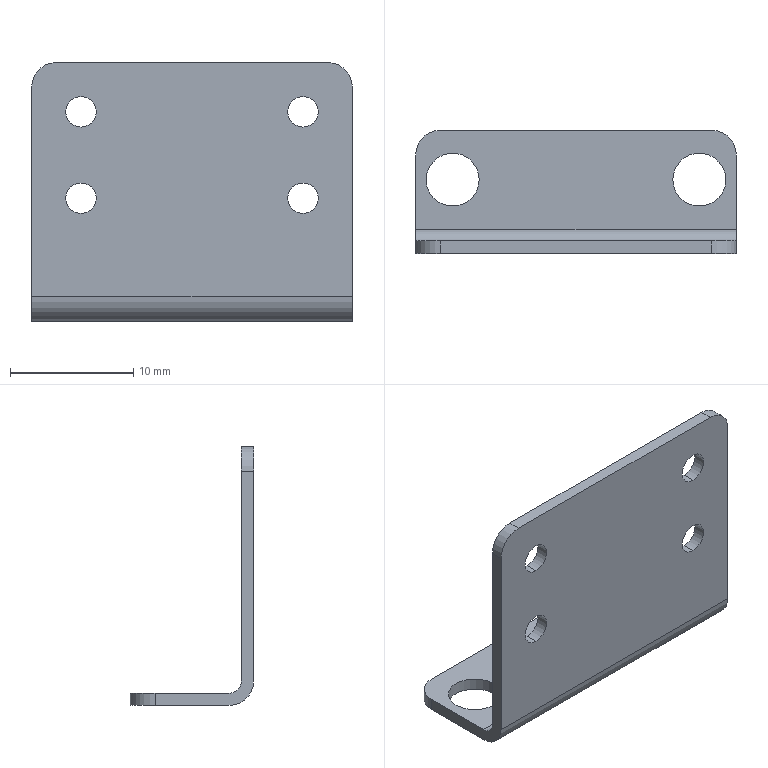Part | SolidWorks | features BaseBody 1 | 1 solid | 26 faces | box 26 x 10 x 21 mm | volume 711.787 mm3 | cylinder 18 | plane 8 | commonest cylinder face diameters 2.459 x8 4 x5 4.3 x4 2 x1
STEP:
#1=CARTESIAN_POINT('',(225.979,1907.294,-6.729));
#2=VERTEX_POINT('',#1);
#3=CARTESIAN_POINT('',(225.979,1907.294,-4.271));
#4=VERTEX_POINT('',#3);
#5=CARTESIAN_POINT('',(225.979,1907.294,-5.5));
#6=DIRECTION('',(0.,1.,0.));
#7=DIRECTION('',(0.,0.,1.));
#8=AXIS2_PLACEMENT_3D('',#5,#6,#7);
#9=CIRCLE('',#8,1.229);
#10=EDGE_CURVE('',#2,#4,#9,.T.);
#11=ORIENTED_EDGE('',*,*,#10,.F.);
#12=CARTESIAN_POINT('',(225.979,1908.294,-6.729));
#13=VERTEX_POINT('',#12);
#14=CARTESIAN_POINT('',(225.979,1873.408,-6.729));
#15=DIRECTION('',(0.,1.,0.));
#16=VECTOR('',#15,1000.);
#17=LINE('',#14,#16);
#18=EDGE_CURVE('',#2,#13,#17,.T.);
#19=ORIENTED_EDGE('',*,*,#18,.T.);
#20=CARTESIAN_POINT('',(225.979,1908.294,-4.271));
#21=VERTEX_POINT('',#20);
#22=CARTESIAN_POINT('',(225.979,1908.294,-5.5));
#23=DIRECTION('',(0.,-1.,0.));
#24=DIRECTION('',(0.,0.,1.));
#25=AXIS2_PLACEMENT_3D('',#22,#23,#24);
#26=CIRCLE('',#25,1.229);
#27=EDGE_CURVE('',#21,#13,#26,.T.);
#28=ORIENTED_EDGE('',*,*,#27,.F.);
#29=CARTESIAN_POINT('',(225.979,1873.408,-4.271));
#30=DIRECTION('',(0.,1.,0.));
#31=VECTOR('',#30,1000.);
#32=LINE('',#29,#31);
#33=EDGE_CURVE('',#4,#21,#32,.T.);
#34=ORIENTED_EDGE('',*,*,#33,.F.);
#35=EDGE_LOOP('',(#11,#19,#28,#34));
#36=FACE_OUTER_BOUND('',#35,.T.);
#37=CARTESIAN_POINT('',(225.979,1873.408,-5.5));
#38=DIRECTION('',(0.,1.,0.));
#39=DIRECTION('',(0.,0.,1.));
#40=AXIS2_PLACEMENT_3D('',#37,#38,#39);
#41=CYLINDRICAL_SURFACE('',#40,1.229);
#42=ADVANCED_FACE('',(#36),#41,.F.);
#43=CARTESIAN_POINT('',(207.979,1907.294,-13.729));
#44=VERTEX_POINT('',#43);
#45=CARTESIAN_POINT('',(207.979,1907.294,-11.271));
#46=VERTEX_POINT('',#45);
#47=CARTESIAN_POINT('',(207.979,1907.294,-12.5));
#48=DIRECTION('',(0.,1.,0.));
#49=DIRECTION('',(0.,0.,1.));
#50=AXIS2_PLACEMENT_3D('',#47,#48,#49);
#51=CIRCLE('',#50,1.229);
#52=EDGE_CURVE('',#44,#46,#51,.T.);
#53=ORIENTED_EDGE('',*,*,#52,.F.);
#54=CARTESIAN_POINT('',(207.979,1908.294,-13.729));
#55=VERTEX_POINT('',#54);
#56=CARTESIAN_POINT('',(207.979,1873.408,-13.729));
#57=DIRECTION('',(0.,1.,0.));
#58=VECTOR('',#57,1000.);
#59=LINE('',#56,#58);
#60=EDGE_CURVE('',#44,#55,#59,.T.);
#61=ORIENTED_EDGE('',*,*,#60,.T.);
#62=CARTESIAN_POINT('',(207.979,1908.294,-11.271));
#63=VERTEX_POINT('',#62);
#64=CARTESIAN_POINT('',(207.979,1908.294,-12.5));
#65=DIRECTION('',(0.,-1.,0.));
#66=DIRECTION('',(0.,0.,1.));
#67=AXIS2_PLACEMENT_3D('',#64,#65,#66);
#68=CIRCLE('',#67,1.229);
#69=EDGE_CURVE('',#63,#55,#68,.T.);
#70=ORIENTED_EDGE('',*,*,#69,.F.);
#71=CARTESIAN_POINT('',(207.979,1873.408,-11.271));
#72=DIRECTION('',(0.,1.,0.));
#73=VECTOR('',#72,1000.);
#74=LINE('',#71,#73);
#75=EDGE_CURVE('',#46,#63,#74,.T.);
#76=ORIENTED_EDGE('',*,*,#75,.F.);
#77=EDGE_LOOP('',(#53,#61,#70,#76));
#78=FACE_OUTER_BOUND('',#77,.T.);
#79=CARTESIAN_POINT('',(207.979,1873.408,-12.5));
#80=DIRECTION('',(0.,1.,0.));
#81=DIRECTION('',(0.,0.,1.));
#82=AXIS2_PLACEMENT_3D('',#79,#80,#81);
#83=CYLINDRICAL_SURFACE('',#82,1.229);
#84=ADVANCED_FACE('',(#78),#83,.F.);
#85=CARTESIAN_POINT('',(207.979,1907.294,-6.729));
#86=VERTEX_POINT('',#85);
#87=CARTESIAN_POINT('',(207.979,1907.294,-4.271));
#88=VERTEX_POINT('',#87);
#89=CARTESIAN_POINT('',(207.979,1907.294,-5.5));
#90=DIRECTION('',(0.,1.,0.));
#91=DIRECTION('',(0.,0.,1.));
#92=AXIS2_PLACEMENT_3D('',#89,#90,#91);
#93=CIRCLE('',#92,1.229);
#94=EDGE_CURVE('',#86,#88,#93,.T.);
#95=ORIENTED_EDGE('',*,*,#94,.F.);
#96=CARTESIAN_POINT('',(207.979,1908.294,-6.729));
#97=VERTEX_POINT('',#96);
#98=CARTESIAN_POINT('',(207.979,1873.408,-6.729));
#99=DIRECTION('',(0.,1.,0.));
#100=VECTOR('',#99,1000.);
#101=LINE('',#98,#100);
#102=EDGE_CURVE('',#86,#97,#101,.T.);
#103=ORIENTED_EDGE('',*,*,#102,.T.);
#104=CARTESIAN_POINT('',(207.979,1908.294,-4.271));
#105=VERTEX_POINT('',#104);
#106=CARTESIAN_POINT('',(207.979,1908.294,-5.5));
#107=DIRECTION('',(0.,-1.,0.));
#108=DIRECTION('',(0.,0.,1.));
#109=AXIS2_PLACEMENT_3D('',#106,#107,#108);
#110=CIRCLE('',#109,1.229);
#111=EDGE_CURVE('',#105,#97,#110,.T.);
#112=ORIENTED_EDGE('',*,*,#111,.F.);
#113=CARTESIAN_POINT('',(207.979,1873.408,-4.271));
#114=DIRECTION('',(0.,1.,0.));
#115=VECTOR('',#114,1000.);
#116=LINE('',#113,#115);
#117=EDGE_CURVE('',#88,#105,#116,.T.);
#118=ORIENTED_EDGE('',*,*,#117,.F.);
#119=EDGE_LOOP('',(#95,#103,#112,#118));
#120=FACE_OUTER_BOUND('',#119,.T.);
#121=CARTESIAN_POINT('',(207.979,1873.408,-5.5));
#122=DIRECTION('',(0.,1.,0.));
#123=DIRECTION('',(0.,0.,1.));
#124=AXIS2_PLACEMENT_3D('',#121,#122,#123);
#125=CYLINDRICAL_SURFACE('',#124,1.229);
#126=ADVANCED_FACE('',(#120),#125,.F.);
#127=CARTESIAN_POINT('',(225.979,1907.294,-13.729));
#128=VERTEX_POINT('',#127);
#129=CARTESIAN_POINT('',(225.979,1907.294,-11.271));
#130=VERTEX_POINT('',#129);
#131=CARTESIAN_POINT('',(225.979,1907.294,-12.5));
#132=DIRECTION('',(0.,1.,0.));
#133=DIRECTION('',(0.,0.,1.));
#134=AXIS2_PLACEMENT_3D('',#131,#132,#133);
#135=CIRCLE('',#134,1.229);
#136=EDGE_CURVE('',#128,#130,#135,.T.);
#137=ORIENTED_EDGE('',*,*,#136,.F.);
#138=CARTESIAN_POINT('',(225.979,1908.294,-13.729));
#139=VERTEX_POINT('',#138);
#140=CARTESIAN_POINT('',(225.979,1873.408,-13.729));
#141=DIRECTION('',(0.,1.,0.));
#142=VECTOR('',#141,1000.);
#143=LINE('',#140,#142);
#144=EDGE_CURVE('',#128,#139,#143,.T.);
#145=ORIENTED_EDGE('',*,*,#144,.T.);
#146=CARTESIAN_POINT('',(225.979,1908.294,-11.271));
#147=VERTEX_POINT('',#146);
#148=CARTESIAN_POINT('',(225.979,1908.294,-12.5));
#149=DIRECTION('',(0.,-1.,0.));
#150=DIRECTION('',(0.,0.,1.));
#151=AXIS2_PLACEMENT_3D('',#148,#149,#150);
#152=CIRCLE('',#151,1.229);
#153=EDGE_CURVE('',#147,#139,#152,.T.);
#154=ORIENTED_EDGE('',*,*,#153,.F.);
#155=CARTESIAN_POINT('',(225.979,1873.408,-11.271));
#156=DIRECTION('',(0.,1.,0.));
#157=VECTOR('',#156,1000.);
#158=LINE('',#155,#157);
#159=EDGE_CURVE('',#130,#147,#158,.T.);
#160=ORIENTED_EDGE('',*,*,#159,.F.);
#161=EDGE_LOOP('',(#137,#145,#154,#160));
#162=FACE_OUTER_BOUND('',#161,.T.);
#163=CARTESIAN_POINT('',(225.979,1873.408,-12.5));
#164=DIRECTION('',(0.,1.,0.));
#165=DIRECTION('',(0.,0.,1.));
#166=AXIS2_PLACEMENT_3D('',#163,#164,#165);
#167=CYLINDRICAL_SURFACE('',#166,1.229);
#168=ADVANCED_FACE('',(#162),#167,.F.);
#169=CARTESIAN_POINT('',(209.129,1913.294,-22.5));
#170=VERTEX_POINT('',#169);
#171=CARTESIAN_POINT('',(204.829,1913.294,-22.5));
#172=VERTEX_POINT('',#171);
#173=CARTESIAN_POINT('',(206.979,1913.294,-22.5));
#174=DIRECTION('',(0.,0.,-1.));
#175=DIRECTION('',(1.,0.,0.));
#176=AXIS2_PLACEMENT_3D('',#173,#174,#175);
#177=CIRCLE('',#176,2.15);
#178=EDGE_CURVE('',#170,#172,#177,.T.);
#179=ORIENTED_EDGE('',*,*,#178,.T.);
#180=CARTESIAN_POINT('',(204.829,1913.294,-21.5));
#181=VERTEX_POINT('',#180);
#182=CARTESIAN_POINT('',(204.829,1913.294,-49.375));
#183=DIRECTION('',(0.,0.,1.));
#184=VECTOR('',#183,1000.);
#185=LINE('',#182,#184);
#186=EDGE_CURVE('',#172,#181,#185,.T.);
#187=ORIENTED_EDGE('',*,*,#186,.T.);
#188=CARTESIAN_POINT('',(209.129,1913.294,-21.5));
#189=VERTEX_POINT('',#188);
#190=CARTESIAN_POINT('',(206.979,1913.294,-21.5));
#191=DIRECTION('',(0.,0.,-1.));
#192=DIRECTION('',(1.,0.,0.));
#193=AXIS2_PLACEMENT_3D('',#190,#191,#192);
#194=CIRCLE('',#193,2.15);
#195=EDGE_CURVE('',#189,#181,#194,.T.);
#196=ORIENTED_EDGE('',*,*,#195,.F.);
#197=CARTESIAN_POINT('',(209.129,1913.294,-49.375));
#198=DIRECTION('',(0.,0.,1.));
#199=VECTOR('',#198,1000.);
#200=LINE('',#197,#199);
#201=EDGE_CURVE('',#170,#189,#200,.T.);
#202=ORIENTED_EDGE('',*,*,#201,.F.);
#203=EDGE_LOOP('',(#179,#187,#196,#202));
#204=FACE_OUTER_BOUND('',#203,.T.);
#205=CARTESIAN_POINT('',(206.979,1913.294,-49.375));
#206=DIRECTION('',(0.,0.,1.));
#207=DIRECTION('',(1.,0.,0.));
#208=AXIS2_PLACEMENT_3D('',#205,#206,#207);
#209=CYLINDRICAL_SURFACE('',#208,2.15);
#210=ADVANCED_FACE('',(#204),#209,.F.);
#211=CARTESIAN_POINT('',(229.129,1913.294,-22.5));
#212=VERTEX_POINT('',#211);
#213=CARTESIAN_POINT('',(224.829,1913.294,-22.5));
#214=VERTEX_POINT('',#213);
#215=CARTESIAN_POINT('',(226.979,1913.294,-22.5));
#216=DIRECTION('',(0.,0.,-1.));
#217=DIRECTION('',(1.,0.,0.));
#218=AXIS2_PLACEMENT_3D('',#215,#216,#217);
#219=CIRCLE('',#218,2.15);
#220=EDGE_CURVE('',#212,#214,#219,.T.);
#221=ORIENTED_EDGE('',*,*,#220,.T.);
#222=CARTESIAN_POINT('',(224.829,1913.294,-21.5));
#223=VERTEX_POINT('',#222);
#224=CARTESIAN_POINT('',(224.829,1913.294,-49.375));
#225=DIRECTION('',(0.,0.,1.));
#226=VECTOR('',#225,1000.);
#227=LINE('',#224,#226);
#228=EDGE_CURVE('',#214,#223,#227,.T.);
#229=ORIENTED_EDGE('',*,*,#228,.T.);
#230=CARTESIAN_POINT('',(229.129,1913.294,-21.5));
#231=VERTEX_POINT('',#230);
#232=CARTESIAN_POINT('',(226.979,1913.294,-21.5));
#233=DIRECTION('',(0.,0.,-1.));
#234=DIRECTION('',(1.,0.,0.));
#235=AXIS2_PLACEMENT_3D('',#232,#233,#234);
#236=CIRCLE('',#235,2.15);
#237=EDGE_CURVE('',#231,#223,#236,.T.);
#238=ORIENTED_EDGE('',*,*,#237,.F.);
#239=CARTESIAN_POINT('',(229.129,1913.294,-49.375));
#240=DIRECTION('',(0.,0.,1.));
#241=VECTOR('',#240,1000.);
#242=LINE('',#239,#241);
#243=EDGE_CURVE('',#212,#231,#242,.T.);
#244=ORIENTED_EDGE('',*,*,#243,.F.);
#245=EDGE_LOOP('',(#221,#229,#238,#244));
#246=FACE_OUTER_BOUND('',#245,.T.);
#247=CARTESIAN_POINT('',(226.979,1913.294,-49.375));
#248=DIRECTION('',(0.,0.,1.));
#249=DIRECTION('',(1.,0.,0.));
#250=AXIS2_PLACEMENT_3D('',#247,#248,#249);
#251=CYLINDRICAL_SURFACE('',#250,2.15);
#252=ADVANCED_FACE('',(#246),#251,.F.);
#253=CARTESIAN_POINT('',(225.979,1907.294,-5.5));
#254=DIRECTION('',(0.,1.,0.));
#255=DIRECTION('',(0.,0.,1.));
#256=AXIS2_PLACEMENT_3D('',#253,#254,#255);
#257=CIRCLE('',#256,1.229);
#258=EDGE_CURVE('',#4,#2,#257,.T.);
#259=ORIENTED_EDGE('',*,*,#258,.T.);
#260=ORIENTED_EDGE('',*,*,#10,.T.);
#261=EDGE_LOOP('',(#259,#260));
#262=FACE_BOUND('',#261,.T.);
#263=CARTESIAN_POINT('',(207.979,1907.294,-12.5));
#264=DIRECTION('',(0.,1.,0.));
#265=DIRECTION('',(0.,0.,1.));
#266=AXIS2_PLACEMENT_3D('',#263,#264,#265);
#267=CIRCLE('',#266,1.229);
#268=EDGE_CURVE('',#46,#44,#267,.T.);
#269=ORIENTED_EDGE('',*,*,#268,.T.);
#270=ORIENTED_EDGE('',*,*,#52,.T.);
#271=EDGE_LOOP('',(#269,#270));
#272=FACE_BOUND('',#271,.T.);
#273=CARTESIAN_POINT('',(207.979,1907.294,-5.5));
#274=DIRECTION('',(0.,1.,0.));
#275=DIRECTION('',(0.,0.,1.));
#276=AXIS2_PLACEMENT_3D('',#273,#274,#275);
#277=CIRCLE('',#276,1.229);
#278=EDGE_CURVE('',#88,#86,#277,.T.);
#279=ORIENTED_EDGE('',*,*,#278,.T.);
#280=ORIENTED_EDGE('',*,*,#94,.T.);
#281=EDGE_LOOP('',(#279,#280));
#282=FACE_BOUND('',#281,.T.);
#283=CARTESIAN_POINT('',(225.979,1907.294,-12.5));
#284=DIRECTION('',(0.,1.,0.));
#285=DIRECTION('',(0.,0.,1.));
#286=AXIS2_PLACEMENT_3D('',#283,#284,#285);
#287=CIRCLE('',#286,1.229);
#288=EDGE_CURVE('',#130,#128,#287,.T.);
#289=ORIENTED_EDGE('',*,*,#288,.T.);
#290=ORIENTED_EDGE('',*,*,#136,.T.);
#291=EDGE_LOOP('',(#289,#290));
#292=FACE_BOUND('',#291,.T.);
#293=CARTESIAN_POINT('',(229.979,1907.294,-20.5));
#294=VERTEX_POINT('',#293);
#295=CARTESIAN_POINT('',(229.979,1907.294,-3.5));
#296=VERTEX_POINT('',#295);
#297=CARTESIAN_POINT('',(229.979,1907.294,-22.5));
#298=DIRECTION('',(0.,0.,1.));
#299=VECTOR('',#298,1000.);
#300=LINE('',#297,#299);
#301=EDGE_CURVE('',#294,#296,#300,.T.);
#302=ORIENTED_EDGE('',*,*,#301,.T.);
#303=CARTESIAN_POINT('',(227.979,1907.294,-1.5));
#304=VERTEX_POINT('',#303);
#305=CARTESIAN_POINT('',(227.979,1907.294,-3.5));
#306=DIRECTION('',(0.,-1.,0.));
#307=DIRECTION('',(0.,0.,1.));
#308=AXIS2_PLACEMENT_3D('',#305,#306,#307);
#309=CIRCLE('',#308,2.);
#310=EDGE_CURVE('',#296,#304,#309,.T.);
#311=ORIENTED_EDGE('',*,*,#310,.T.);
#312=CARTESIAN_POINT('',(205.979,1907.294,-1.5));
#313=VERTEX_POINT('',#312);
#314=CARTESIAN_POINT('',(203.979,1907.294,-1.5));
#315=DIRECTION('',(-1.,0.,0.));
#316=VECTOR('',#315,1000.);
#317=LINE('',#314,#316);
#318=EDGE_CURVE('',#304,#313,#317,.T.);
#319=ORIENTED_EDGE('',*,*,#318,.T.);
#320=CARTESIAN_POINT('',(203.979,1907.294,-3.5));
#321=VERTEX_POINT('',#320);
#322=CARTESIAN_POINT('',(205.979,1907.294,-3.5));
#323=DIRECTION('',(0.,-1.,0.));
#324=DIRECTION('',(0.,0.,-1.));
#325=AXIS2_PLACEMENT_3D('',#322,#323,#324);
#326=CIRCLE('',#325,2.);
#327=EDGE_CURVE('',#313,#321,#326,.T.);
#328=ORIENTED_EDGE('',*,*,#327,.T.);
#329=CARTESIAN_POINT('',(203.979,1907.294,-20.5));
#330=VERTEX_POINT('',#329);
#331=CARTESIAN_POINT('',(203.979,1907.294,-22.5));
#332=DIRECTION('',(0.,0.,-1.));
#333=VECTOR('',#332,1000.);
#334=LINE('',#331,#333);
#335=EDGE_CURVE('',#321,#330,#334,.T.);
#336=ORIENTED_EDGE('',*,*,#335,.T.);
#337=CARTESIAN_POINT('',(203.979,1907.294,-20.5));
#338=DIRECTION('',(1.,0.,0.));
#339=VECTOR('',#338,1000.);
#340=LINE('',#337,#339);
#341=EDGE_CURVE('',#330,#294,#340,.T.);
#342=ORIENTED_EDGE('',*,*,#341,.T.);
#343=EDGE_LOOP('',(#302,#311,#319,#328,#336,#342));
#344=FACE_OUTER_BOUND('',#343,.T.);
#345=CARTESIAN_POINT('',(203.979,1907.294,-22.5));
#346=DIRECTION('',(0.,-1.,0.));
#347=DIRECTION('',(0.,0.,-1.));
#348=AXIS2_PLACEMENT_3D('',#345,#346,#347);
#349=PLANE('',#348);
#350=ADVANCED_FACE('',(#262,#272,#282,#292,#344),#349,.T.);
#351=ORIENTED_EDGE('',*,*,#18,.F.);
#352=ORIENTED_EDGE('',*,*,#258,.F.);
#353=ORIENTED_EDGE('',*,*,#33,.T.);
#354=CARTESIAN_POINT('',(225.979,1908.294,-5.5));
#355=DIRECTION('',(0.,-1.,0.));
#356=DIRECTION('',(0.,0.,1.));
#357=AXIS2_PLACEMENT_3D('',#354,#355,#356);
#358=CIRCLE('',#357,1.229);
#359=EDGE_CURVE('',#13,#21,#358,.T.);
#360=ORIENTED_EDGE('',*,*,#359,.F.);
#361=EDGE_LOOP('',(#351,#352,#353,#360));
#362=FACE_OUTER_BOUND('',#361,.T.);
#363=CARTESIAN_POINT('',(225.979,1873.408,-5.5));
#364=DIRECTION('',(0.,1.,0.));
#365=DIRECTION('',(0.,0.,1.));
#366=AXIS2_PLACEMENT_3D('',#363,#364,#365);
#367=CYLINDRICAL_SURFACE('',#366,1.229);
#368=ADVANCED_FACE('',(#362),#367,.F.);
#369=ORIENTED_EDGE('',*,*,#60,.F.);
#370=ORIENTED_EDGE('',*,*,#268,.F.);
#371=ORIENTED_EDGE('',*,*,#75,.T.);
#372=CARTESIAN_POINT('',(207.979,1908.294,-12.5));
#373=DIRECTION('',(0.,-1.,0.));
#374=DIRECTION('',(0.,0.,1.));
#375=AXIS2_PLACEMENT_3D('',#372,#373,#374);
#376=CIRCLE('',#375,1.229);
#377=EDGE_CURVE('',#55,#63,#376,.T.);
#378=ORIENTED_EDGE('',*,*,#377,.F.);
#379=EDGE_LOOP('',(#369,#370,#371,#378));
#380=FACE_OUTER_BOUND('',#379,.T.);
#381=CARTESIAN_POINT('',(207.979,1873.408,-12.5));
#382=DIRECTION('',(0.,1.,0.));
#383=DIRECTION('',(0.,0.,1.));
#384=AXIS2_PLACEMENT_3D('',#381,#382,#383);
#385=CYLINDRICAL_SURFACE('',#384,1.229);
#386=ADVANCED_FACE('',(#380),#385,.F.);
#387=ORIENTED_EDGE('',*,*,#102,.F.);
#388=ORIENTED_EDGE('',*,*,#278,.F.);
#389=ORIENTED_EDGE('',*,*,#117,.T.);
#390=CARTESIAN_POINT('',(207.979,1908.294,-5.5));
#391=DIRECTION('',(0.,-1.,0.));
#392=DIRECTION('',(0.,0.,1.));
#393=AXIS2_PLACEMENT_3D('',#390,#391,#392);
#394=CIRCLE('',#393,1.229);
#395=EDGE_CURVE('',#97,#105,#394,.T.);
#396=ORIENTED_EDGE('',*,*,#395,.F.);
#397=EDGE_LOOP('',(#387,#388,#389,#396));
#398=FACE_OUTER_BOUND('',#397,.T.);
#399=CARTESIAN_POINT('',(207.979,1873.408,-5.5));
#400=DIRECTION('',(0.,1.,0.));
#401=DIRECTION('',(0.,0.,1.));
#402=AXIS2_PLACEMENT_3D('',#399,#400,#401);
#403=CYLINDRICAL_SURFACE('',#402,1.229);
#404=ADVANCED_FACE('',(#398),#403,.F.);
#405=ORIENTED_EDGE('',*,*,#144,.F.);
#406=ORIENTED_EDGE('',*,*,#288,.F.);
#407=ORIENTED_EDGE('',*,*,#159,.T.);
#408=CARTESIAN_POINT('',(225.979,1908.294,-12.5));
#409=DIRECTION('',(0.,-1.,0.));
#410=DIRECTION('',(0.,0.,1.));
#411=AXIS2_PLACEMENT_3D('',#408,#409,#410);
#412=CIRCLE('',#411,1.229);
#413=EDGE_CURVE('',#139,#147,#412,.T.);
#414=ORIENTED_EDGE('',*,*,#413,.F.);
#415=EDGE_LOOP('',(#405,#406,#407,#414));
#416=FACE_OUTER_BOUND('',#415,.T.);
#417=CARTESIAN_POINT('',(225.979,1873.408,-12.5));
#418=DIRECTION('',(0.,1.,0.));
#419=DIRECTION('',(0.,0.,1.));
#420=AXIS2_PLACEMENT_3D('',#417,#418,#419);
#421=CYLINDRICAL_SURFACE('',#420,1.229);
#422=ADVANCED_FACE('',(#416),#421,.F.);
#423=CARTESIAN_POINT('',(227.979,1908.294,-1.5));
#424=VERTEX_POINT('',#423);
#425=CARTESIAN_POINT('',(227.979,1907.544,-1.5));
#426=DIRECTION('',(0.,-1.,0.));
#427=VECTOR('',#426,1000.);
#428=LINE('',#425,#427);
#429=EDGE_CURVE('',#424,#304,#428,.T.);
#430=ORIENTED_EDGE('',*,*,#429,.T.);
#431=ORIENTED_EDGE('',*,*,#310,.F.);
#432=CARTESIAN_POINT('',(229.979,1908.294,-3.5));
#433=VERTEX_POINT('',#432);
#434=CARTESIAN_POINT('',(229.979,1907.544,-3.5));
#435=DIRECTION('',(0.,1.,0.));
#436=VECTOR('',#435,1000.);
#437=LINE('',#434,#436);
#438=EDGE_CURVE('',#296,#433,#437,.T.);
#439=ORIENTED_EDGE('',*,*,#438,.T.);
#440=CARTESIAN_POINT('',(227.979,1908.294,-3.5));
#441=DIRECTION('',(0.,-1.,0.));
#442=DIRECTION('',(0.,0.,1.));
#443=AXIS2_PLACEMENT_3D('',#440,#441,#442);
#444=CIRCLE('',#443,2.);
#445=EDGE_CURVE('',#433,#424,#444,.T.);
#446=ORIENTED_EDGE('',*,*,#445,.T.);
#447=EDGE_LOOP('',(#430,#431,#439,#446));
#448=FACE_OUTER_BOUND('',#447,.T.);
#449=CARTESIAN_POINT('',(227.979,1907.544,-3.5));
#450=DIRECTION('',(0.,1.,0.));
#451=DIRECTION('',(0.,0.,1.));
#452=AXIS2_PLACEMENT_3D('',#449,#450,#451);
#453=CYLINDRICAL_SURFACE('',#452,2.);
#454=ADVANCED_FACE('',(#448),#453,.T.);
#455=CARTESIAN_POINT('',(229.979,1915.294,-22.5));
#456=VERTEX_POINT('',#455);
#457=CARTESIAN_POINT('',(229.979,1909.294,-22.5));
#458=VERTEX_POINT('',#457);
#459=CARTESIAN_POINT('',(229.979,1907.794,-22.5));
#460=DIRECTION('',(0.,-1.,0.));
#461=VECTOR('',#460,1000.);
#462=LINE('',#459,#461);
#463=EDGE_CURVE('',#456,#458,#462,.T.);
#464=ORIENTED_EDGE('',*,*,#463,.F.);
#465=CARTESIAN_POINT('',(229.979,1915.294,-21.5));
#466=VERTEX_POINT('',#465);
#467=CARTESIAN_POINT('',(229.979,1915.294,-12.));
#468=DIRECTION('',(0.,0.,-1.));
#469=VECTOR('',#468,1000.);
#470=LINE('',#467,#469);
#471=EDGE_CURVE('',#466,#456,#470,.T.);
#472=ORIENTED_EDGE('',*,*,#471,.F.);
#473=CARTESIAN_POINT('',(229.979,1909.294,-21.5));
#474=VERTEX_POINT('',#473);
#475=CARTESIAN_POINT('',(229.979,1907.794,-21.5));
#476=DIRECTION('',(0.,1.,0.));
#477=VECTOR('',#476,1000.);
#478=LINE('',#475,#477);
#479=EDGE_CURVE('',#474,#466,#478,.T.);
#480=ORIENTED_EDGE('',*,*,#479,.F.);
#481=CARTESIAN_POINT('',(229.979,1908.294,-20.5));
#482=VERTEX_POINT('',#481);
#483=CARTESIAN_POINT('',(229.979,1909.294,-20.5));
#484=DIRECTION('',(1.,0.,0.));
#485=DIRECTION('',(0.,0.,1.));
#486=AXIS2_PLACEMENT_3D('',#483,#484,#485);
#487=CIRCLE('',#486,1.);
#488=EDGE_CURVE('',#482,#474,#487,.T.);
#489=ORIENTED_EDGE('',*,*,#488,.F.);
#490=CARTESIAN_POINT('',(229.979,1908.294,-12.));
#491=DIRECTION('',(0.,0.,-1.));
#492=VECTOR('',#491,1000.);
#493=LINE('',#490,#492);
#494=EDGE_CURVE('',#433,#482,#493,.T.);
#495=ORIENTED_EDGE('',*,*,#494,.F.);
#496=ORIENTED_EDGE('',*,*,#438,.F.);
#497=ORIENTED_EDGE('',*,*,#301,.F.);
#498=CARTESIAN_POINT('',(229.979,1909.294,-20.5));
#499=DIRECTION('',(-1.,0.,0.));
#500=DIRECTION('',(0.,0.,1.));
#501=AXIS2_PLACEMENT_3D('',#498,#499,#500);
#502=CIRCLE('',#501,2.);
#503=EDGE_CURVE('',#458,#294,#502,.T.);
#504=ORIENTED_EDGE('',*,*,#503,.F.);
#505=EDGE_LOOP('',(#464,#472,#480,#489,#495,#496,#497,#504));
#506=FACE_OUTER_BOUND('',#505,.T.);
#507=CARTESIAN_POINT('',(229.979,1907.794,-12.));
#508=DIRECTION('',(-1.,0.,0.));
#509=DIRECTION('',(0.,0.,1.));
#510=AXIS2_PLACEMENT_3D('',#507,#508,#509);
#511=PLANE('',#510);
#512=ADVANCED_FACE('',(#506),#511,.F.);
#513=CARTESIAN_POINT('',(203.979,1909.294,-22.5));
#514=VERTEX_POINT('',#513);
#515=CARTESIAN_POINT('',(203.979,1909.294,-20.5));
#516=DIRECTION('',(1.,0.,0.));
#517=DIRECTION('',(0.,0.,1.));
#518=AXIS2_PLACEMENT_3D('',#515,#516,#517);
#519=CIRCLE('',#518,2.);
#520=EDGE_CURVE('',#330,#514,#519,.T.);
#521=ORIENTED_EDGE('',*,*,#520,.T.);
#522=CARTESIAN_POINT('',(216.979,1909.294,-22.5));
#523=DIRECTION('',(1.,0.,0.));
#524=VECTOR('',#523,1000.);
#525=LINE('',#522,#524);
#526=EDGE_CURVE('',#514,#458,#525,.T.);
#527=ORIENTED_EDGE('',*,*,#526,.T.);
#528=ORIENTED_EDGE('',*,*,#503,.T.);
#529=ORIENTED_EDGE('',*,*,#341,.F.);
#530=EDGE_LOOP('',(#521,#527,#528,#529));
#531=FACE_OUTER_BOUND('',#530,.T.);
#532=CARTESIAN_POINT('',(216.979,1909.294,-20.5));
#533=DIRECTION('',(-1.,0.,0.));
#534=DIRECTION('',(0.,0.,1.));
#535=AXIS2_PLACEMENT_3D('',#532,#533,#534);
#536=CYLINDRICAL_SURFACE('',#535,2.);
#537=ADVANCED_FACE('',(#531),#536,.T.);
#538=CARTESIAN_POINT('',(203.979,1915.294,-22.5));
#539=VERTEX_POINT('',#538);
#540=CARTESIAN_POINT('',(203.979,1907.794,-22.5));
#541=DIRECTION('',(0.,-1.,0.));
#542=VECTOR('',#541,1000.);
#543=LINE('',#540,#542);
#544=EDGE_CURVE('',#539,#514,#543,.T.);
#545=ORIENTED_EDGE('',*,*,#544,.T.);
#546=ORIENTED_EDGE('',*,*,#520,.F.);
#547=ORIENTED_EDGE('',*,*,#335,.F.);
#548=CARTESIAN_POINT('',(203.979,1908.294,-3.5));
#549=VERTEX_POINT('',#548);
#550=CARTESIAN_POINT('',(203.979,1907.794,-3.5));
#551=DIRECTION('',(0.,1.,0.));
#552=VECTOR('',#551,1000.);
#553=LINE('',#550,#552);
#554=EDGE_CURVE('',#321,#549,#553,.T.);
#555=ORIENTED_EDGE('',*,*,#554,.T.);
#556=CARTESIAN_POINT('',(203.979,1908.294,-20.5));
#557=VERTEX_POINT('',#556);
#558=CARTESIAN_POINT('',(203.979,1908.294,-12.));
#559=DIRECTION('',(0.,0.,-1.));
#560=VECTOR('',#559,1000.);
#561=LINE('',#558,#560);
#562=EDGE_CURVE('',#549,#557,#561,.T.);
#563=ORIENTED_EDGE('',*,*,#562,.T.);
#564=CARTESIAN_POINT('',(203.979,1909.294,-21.5));
#565=VERTEX_POINT('',#564);
#566=CARTESIAN_POINT('',(203.979,1909.294,-20.5));
#567=DIRECTION('',(1.,0.,0.));
#568=DIRECTION('',(0.,0.,1.));
#569=AXIS2_PLACEMENT_3D('',#566,#567,#568);
#570=CIRCLE('',#569,1.);
#571=EDGE_CURVE('',#557,#565,#570,.T.);
#572=ORIENTED_EDGE('',*,*,#571,.T.);
#573=CARTESIAN_POINT('',(203.979,1915.294,-21.5));
#574=VERTEX_POINT('',#573);
#575=CARTESIAN_POINT('',(203.979,1907.794,-21.5));
#576=DIRECTION('',(0.,1.,0.));
#577=VECTOR('',#576,1000.);
#578=LINE('',#575,#577);
#579=EDGE_CURVE('',#565,#574,#578,.T.);
#580=ORIENTED_EDGE('',*,*,#579,.T.);
#581=CARTESIAN_POINT('',(203.979,1915.294,-12.));
#582=DIRECTION('',(0.,0.,-1.));
#583=VECTOR('',#582,1000.);
#584=LINE('',#581,#583);
#585=EDGE_CURVE('',#574,#539,#584,.T.);
#586=ORIENTED_EDGE('',*,*,#585,.T.);
#587=EDGE_LOOP('',(#545,#546,#547,#555,#563,#572,#580,#586));
#588=FACE_OUTER_BOUND('',#587,.T.);
#589=CARTESIAN_POINT('',(203.979,1907.794,-12.));
#590=DIRECTION('',(-1.,0.,0.));
#591=DIRECTION('',(0.,0.,1.));
#592=AXIS2_PLACEMENT_3D('',#589,#590,#591);
#593=PLANE('',#592);
#594=ADVANCED_FACE('',(#588),#593,.T.);
#595=CARTESIAN_POINT('',(205.979,1908.294,-1.5));
#596=VERTEX_POINT('',#595);
#597=CARTESIAN_POINT('',(205.979,1907.544,-1.5));
#598=DIRECTION('',(0.,1.,0.));
#599=VECTOR('',#598,1000.);
#600=LINE('',#597,#599);
#601=EDGE_CURVE('',#313,#596,#600,.T.);
#602=ORIENTED_EDGE('',*,*,#601,.T.);
#603=CARTESIAN_POINT('',(205.979,1908.294,-3.5));
#604=DIRECTION('',(0.,-1.,0.));
#605=DIRECTION('',(0.,0.,-1.));
#606=AXIS2_PLACEMENT_3D('',#603,#604,#605);
#607=CIRCLE('',#606,2.);
#608=EDGE_CURVE('',#596,#549,#607,.T.);
#609=ORIENTED_EDGE('',*,*,#608,.T.);
#610=ORIENTED_EDGE('',*,*,#554,.F.);
#611=ORIENTED_EDGE('',*,*,#327,.F.);
#612=EDGE_LOOP('',(#602,#609,#610,#611));
#613=FACE_OUTER_BOUND('',#612,.T.);
#614=CARTESIAN_POINT('',(205.979,1907.544,-3.5));
#615=DIRECTION('',(0.,-1.,0.));
#616=DIRECTION('',(0.,0.,-1.));
#617=AXIS2_PLACEMENT_3D('',#614,#615,#616);
#618=CYLINDRICAL_SURFACE('',#617,2.);
#619=ADVANCED_FACE('',(#613),#618,.T.);
#620=ORIENTED_EDGE('',*,*,#318,.F.);
#621=ORIENTED_EDGE('',*,*,#429,.F.);
#622=CARTESIAN_POINT('',(203.979,1908.294,-1.5));
#623=DIRECTION('',(-1.,0.,0.));
#624=VECTOR('',#623,1000.);
#625=LINE('',#622,#624);
#626=EDGE_CURVE('',#424,#596,#625,.T.);
#627=ORIENTED_EDGE('',*,*,#626,.T.);
#628=ORIENTED_EDGE('',*,*,#601,.F.);
#629=EDGE_LOOP('',(#620,#621,#627,#628));
#630=FACE_OUTER_BOUND('',#629,.T.);
#631=CARTESIAN_POINT('',(203.979,1907.294,-1.5));
#632=DIRECTION('',(0.,0.,1.));
#633=DIRECTION('',(1.,0.,0.));
#634=AXIS2_PLACEMENT_3D('',#631,#632,#633);
#635=PLANE('',#634);
#636=ADVANCED_FACE('',(#630),#635,.T.);
#637=ORIENTED_EDGE('',*,*,#27,.T.);
#638=ORIENTED_EDGE('',*,*,#359,.T.);
#639=EDGE_LOOP('',(#637,#638));
#640=FACE_BOUND('',#639,.T.);
#641=ORIENTED_EDGE('',*,*,#69,.T.);
#642=ORIENTED_EDGE('',*,*,#377,.T.);
#643=EDGE_LOOP('',(#641,#642));
#644=FACE_BOUND('',#643,.T.);
#645=ORIENTED_EDGE('',*,*,#111,.T.);
#646=ORIENTED_EDGE('',*,*,#395,.T.);
#647=EDGE_LOOP('',(#645,#646));
#648=FACE_BOUND('',#647,.T.);
#649=ORIENTED_EDGE('',*,*,#153,.T.);
#650=ORIENTED_EDGE('',*,*,#413,.T.);
#651=EDGE_LOOP('',(#649,#650));
#652=FACE_BOUND('',#651,.T.);
#653=ORIENTED_EDGE('',*,*,#494,.T.);
#654=CARTESIAN_POINT('',(203.979,1908.294,-20.5));
#655=DIRECTION('',(-1.,0.,0.));
#656=VECTOR('',#655,1000.);
#657=LINE('',#654,#656);
#658=EDGE_CURVE('',#482,#557,#657,.T.);
#659=ORIENTED_EDGE('',*,*,#658,.T.);
#660=ORIENTED_EDGE('',*,*,#562,.F.);
#661=ORIENTED_EDGE('',*,*,#608,.F.);
#662=ORIENTED_EDGE('',*,*,#626,.F.);
#663=ORIENTED_EDGE('',*,*,#445,.F.);
#664=EDGE_LOOP('',(#653,#659,#660,#661,#662,#663));
#665=FACE_OUTER_BOUND('',#664,.T.);
#666=CARTESIAN_POINT('',(203.979,1908.294,-1.5));
#667=DIRECTION('',(0.,1.,0.));
#668=DIRECTION('',(0.,0.,1.));
#669=AXIS2_PLACEMENT_3D('',#666,#667,#668);
#670=PLANE('',#669);
#671=ADVANCED_FACE('',(#640,#644,#648,#652,#665),#670,.T.);
#672=ORIENTED_EDGE('',*,*,#178,.F.);
#673=CARTESIAN_POINT('',(206.979,1913.294,-22.5));
#674=DIRECTION('',(0.,0.,-1.));
#675=DIRECTION('',(1.,0.,0.));
#676=AXIS2_PLACEMENT_3D('',#673,#674,#675);
#677=CIRCLE('',#676,2.15);
#678=EDGE_CURVE('',#172,#170,#677,.T.);
#679=ORIENTED_EDGE('',*,*,#678,.F.);
#680=EDGE_LOOP('',(#672,#679));
#681=FACE_BOUND('',#680,.T.);
#682=ORIENTED_EDGE('',*,*,#220,.F.);
#683=CARTESIAN_POINT('',(226.979,1913.294,-22.5));
#684=DIRECTION('',(0.,0.,-1.));
#685=DIRECTION('',(1.,0.,0.));
#686=AXIS2_PLACEMENT_3D('',#683,#684,#685);
#687=CIRCLE('',#686,2.15);
#688=EDGE_CURVE('',#214,#212,#687,.T.);
#689=ORIENTED_EDGE('',*,*,#688,.F.);
#690=EDGE_LOOP('',(#682,#689));
#691=FACE_BOUND('',#690,.T.);
#692=ORIENTED_EDGE('',*,*,#544,.F.);
#693=CARTESIAN_POINT('',(205.979,1917.294,-22.5));
#694=VERTEX_POINT('',#693);
#695=CARTESIAN_POINT('',(205.979,1915.294,-22.5));
#696=DIRECTION('',(0.,0.,1.));
#697=DIRECTION('',(1.,0.,0.));
#698=AXIS2_PLACEMENT_3D('',#695,#696,#697);
#699=CIRCLE('',#698,2.);
#700=EDGE_CURVE('',#694,#539,#699,.T.);
#701=ORIENTED_EDGE('',*,*,#700,.F.);
#702=CARTESIAN_POINT('',(227.979,1917.294,-22.5));
#703=VERTEX_POINT('',#702);
#704=CARTESIAN_POINT('',(216.979,1917.294,-22.5));
#705=DIRECTION('',(-1.,0.,0.));
#706=VECTOR('',#705,1000.);
#707=LINE('',#704,#706);
#708=EDGE_CURVE('',#703,#694,#707,.T.);
#709=ORIENTED_EDGE('',*,*,#708,.F.);
#710=CARTESIAN_POINT('',(227.979,1915.294,-22.5));
#711=DIRECTION('',(0.,0.,1.));
#712=DIRECTION('',(1.,0.,0.));
#713=AXIS2_PLACEMENT_3D('',#710,#711,#712);
#714=CIRCLE('',#713,2.);
#715=EDGE_CURVE('',#456,#703,#714,.T.);
#716=ORIENTED_EDGE('',*,*,#715,.F.);
#717=ORIENTED_EDGE('',*,*,#463,.T.);
#718=ORIENTED_EDGE('',*,*,#526,.F.);
#719=EDGE_LOOP('',(#692,#701,#709,#716,#717,#718));
#720=FACE_OUTER_BOUND('',#719,.T.);
#721=CARTESIAN_POINT('',(216.979,1912.294,-22.5));
#722=DIRECTION('',(0.,0.,1.));
#723=DIRECTION('',(1.,0.,0.));
#724=AXIS2_PLACEMENT_3D('',#721,#722,#723);
#725=PLANE('',#724);
#726=ADVANCED_FACE('',(#681,#691,#720),#725,.F.);
#727=ORIENTED_EDGE('',*,*,#471,.T.);
#728=ORIENTED_EDGE('',*,*,#715,.T.);
#729=CARTESIAN_POINT('',(227.979,1917.294,-21.5));
#730=VERTEX_POINT('',#729);
#731=CARTESIAN_POINT('',(227.979,1917.294,-17.25));
#732=DIRECTION('',(0.,0.,1.));
#733=VECTOR('',#732,1000.);
#734=LINE('',#731,#733);
#735=EDGE_CURVE('',#703,#730,#734,.T.);
#736=ORIENTED_EDGE('',*,*,#735,.T.);
#737=CARTESIAN_POINT('',(227.979,1915.294,-21.5));
#738=DIRECTION('',(0.,0.,-1.));
#739=DIRECTION('',(1.,0.,0.));
#740=AXIS2_PLACEMENT_3D('',#737,#738,#739);
#741=CIRCLE('',#740,2.);
#742=EDGE_CURVE('',#730,#466,#741,.T.);
#743=ORIENTED_EDGE('',*,*,#742,.T.);
#744=EDGE_LOOP('',(#727,#728,#736,#743));
#745=FACE_OUTER_BOUND('',#744,.T.);
#746=CARTESIAN_POINT('',(227.979,1915.294,-17.25));
#747=DIRECTION('',(0.,0.,1.));
#748=DIRECTION('',(1.,0.,0.));
#749=AXIS2_PLACEMENT_3D('',#746,#747,#748);
#750=CYLINDRICAL_SURFACE('',#749,2.);
#751=ADVANCED_FACE('',(#745),#750,.T.);
#752=ORIENTED_EDGE('',*,*,#237,.T.);
#753=CARTESIAN_POINT('',(226.979,1913.294,-21.5));
#754=DIRECTION('',(0.,0.,-1.));
#755=DIRECTION('',(1.,0.,0.));
#756=AXIS2_PLACEMENT_3D('',#753,#754,#755);
#757=CIRCLE('',#756,2.15);
#758=EDGE_CURVE('',#223,#231,#757,.T.);
#759=ORIENTED_EDGE('',*,*,#758,.T.);
#760=EDGE_LOOP('',(#752,#759));
#761=FACE_BOUND('',#760,.T.);
#762=ORIENTED_EDGE('',*,*,#195,.T.);
#763=CARTESIAN_POINT('',(206.979,1913.294,-21.5));
#764=DIRECTION('',(0.,0.,-1.));
#765=DIRECTION('',(1.,0.,0.));
#766=AXIS2_PLACEMENT_3D('',#763,#764,#765);
#767=CIRCLE('',#766,2.15);
#768=EDGE_CURVE('',#181,#189,#767,.T.);
#769=ORIENTED_EDGE('',*,*,#768,.T.);
#770=EDGE_LOOP('',(#762,#769));
#771=FACE_BOUND('',#770,.T.);
#772=ORIENTED_EDGE('',*,*,#579,.F.);
#773=CARTESIAN_POINT('',(216.979,1909.294,-21.5));
#774=DIRECTION('',(1.,0.,0.));
#775=VECTOR('',#774,1000.);
#776=LINE('',#773,#775);
#777=EDGE_CURVE('',#565,#474,#776,.T.);
#778=ORIENTED_EDGE('',*,*,#777,.T.);
#779=ORIENTED_EDGE('',*,*,#479,.T.);
#780=ORIENTED_EDGE('',*,*,#742,.F.);
#781=CARTESIAN_POINT('',(205.979,1917.294,-21.5));
#782=VERTEX_POINT('',#781);
#783=CARTESIAN_POINT('',(216.979,1917.294,-21.5));
#784=DIRECTION('',(-1.,0.,0.));
#785=VECTOR('',#784,1000.);
#786=LINE('',#783,#785);
#787=EDGE_CURVE('',#730,#782,#786,.T.);
#788=ORIENTED_EDGE('',*,*,#787,.T.);
#789=CARTESIAN_POINT('',(205.979,1915.294,-21.5));
#790=DIRECTION('',(0.,0.,1.));
#791=DIRECTION('',(1.,0.,0.));
#792=AXIS2_PLACEMENT_3D('',#789,#790,#791);
#793=CIRCLE('',#792,2.);
#794=EDGE_CURVE('',#782,#574,#793,.T.);
#795=ORIENTED_EDGE('',*,*,#794,.T.);
#796=EDGE_LOOP('',(#772,#778,#779,#780,#788,#795));
#797=FACE_OUTER_BOUND('',#796,.T.);
#798=CARTESIAN_POINT('',(216.979,1912.294,-21.5));
#799=DIRECTION('',(0.,0.,1.));
#800=DIRECTION('',(1.,0.,0.));
#801=AXIS2_PLACEMENT_3D('',#798,#799,#800);
#802=PLANE('',#801);
#803=ADVANCED_FACE('',(#761,#771,#797),#802,.T.);
#804=ORIENTED_EDGE('',*,*,#571,.F.);
#805=ORIENTED_EDGE('',*,*,#658,.F.);
#806=ORIENTED_EDGE('',*,*,#488,.T.);
#807=ORIENTED_EDGE('',*,*,#777,.F.);
#808=EDGE_LOOP('',(#804,#805,#806,#807));
#809=FACE_OUTER_BOUND('',#808,.T.);
#810=CARTESIAN_POINT('',(216.979,1909.294,-20.5));
#811=DIRECTION('',(-1.,0.,0.));
#812=DIRECTION('',(0.,0.,1.));
#813=AXIS2_PLACEMENT_3D('',#810,#811,#812);
#814=CYLINDRICAL_SURFACE('',#813,1.);
#815=ADVANCED_FACE('',(#809),#814,.F.);
#816=CARTESIAN_POINT('',(205.979,1917.294,-17.25));
#817=DIRECTION('',(0.,0.,-1.));
#818=VECTOR('',#817,1000.);
#819=LINE('',#816,#818);
#820=EDGE_CURVE('',#782,#694,#819,.T.);
#821=ORIENTED_EDGE('',*,*,#820,.T.);
#822=ORIENTED_EDGE('',*,*,#700,.T.);
#823=ORIENTED_EDGE('',*,*,#585,.F.);
#824=ORIENTED_EDGE('',*,*,#794,.F.);
#825=EDGE_LOOP('',(#821,#822,#823,#824));
#826=FACE_OUTER_BOUND('',#825,.T.);
#827=CARTESIAN_POINT('',(205.979,1915.294,-17.25));
#828=DIRECTION('',(0.,0.,1.));
#829=DIRECTION('',(1.,0.,0.));
#830=AXIS2_PLACEMENT_3D('',#827,#828,#829);
#831=CYLINDRICAL_SURFACE('',#830,2.);
#832=ADVANCED_FACE('',(#826),#831,.T.);
#833=ORIENTED_EDGE('',*,*,#186,.F.);
#834=ORIENTED_EDGE('',*,*,#678,.T.);
#835=ORIENTED_EDGE('',*,*,#201,.T.);
#836=ORIENTED_EDGE('',*,*,#768,.F.);
#837=EDGE_LOOP('',(#833,#834,#835,#836));
#838=FACE_OUTER_BOUND('',#837,.T.);
#839=CARTESIAN_POINT('',(206.979,1913.294,-49.375));
#840=DIRECTION('',(0.,0.,1.));
#841=DIRECTION('',(1.,0.,0.));
#842=AXIS2_PLACEMENT_3D('',#839,#840,#841);
#843=CYLINDRICAL_SURFACE('',#842,2.15);
#844=ADVANCED_FACE('',(#838),#843,.F.);
#845=ORIENTED_EDGE('',*,*,#228,.F.);
#846=ORIENTED_EDGE('',*,*,#688,.T.);
#847=ORIENTED_EDGE('',*,*,#243,.T.);
#848=ORIENTED_EDGE('',*,*,#758,.F.);
#849=EDGE_LOOP('',(#845,#846,#847,#848));
#850=FACE_OUTER_BOUND('',#849,.T.);
#851=CARTESIAN_POINT('',(226.979,1913.294,-49.375));
#852=DIRECTION('',(0.,0.,1.));
#853=DIRECTION('',(1.,0.,0.));
#854=AXIS2_PLACEMENT_3D('',#851,#852,#853);
#855=CYLINDRICAL_SURFACE('',#854,2.15);
#856=ADVANCED_FACE('',(#850),#855,.F.);
#857=ORIENTED_EDGE('',*,*,#708,.T.);
#858=ORIENTED_EDGE('',*,*,#820,.F.);
#859=ORIENTED_EDGE('',*,*,#787,.F.);
#860=ORIENTED_EDGE('',*,*,#735,.F.);
#861=EDGE_LOOP('',(#857,#858,#859,#860));
#862=FACE_OUTER_BOUND('',#861,.T.);
#863=CARTESIAN_POINT('',(203.979,1917.294,-22.5));
#864=DIRECTION('',(0.,1.,0.));
#865=DIRECTION('',(0.,0.,1.));
#866=AXIS2_PLACEMENT_3D('',#863,#864,#865);
#867=PLANE('',#866);
#868=ADVANCED_FACE('',(#862),#867,.T.);
#869=CLOSED_SHELL('',(#42,#84,#126,#168,#210,#252,#350,#368,#386,#404,#422,#454,#512,#537,#594,#619,#636,#671,#726,#751,#803,#815,#832,#844,#856,#868));
#870=MANIFOLD_SOLID_BREP('',#869);
#871=CARTESIAN_POINT('',(0.,0.,0.));
#872=DIRECTION('',(0.,0.,1.));
#873=DIRECTION('',(1.,0.,0.));
#874=AXIS2_PLACEMENT_3D('',#871,#872,#873);
#875=(LENGTH_UNIT()NAMED_UNIT(*)SI_UNIT(.MILLI.,.METRE.));
#876=UNCERTAINTY_MEASURE_WITH_UNIT(LENGTH_MEASURE(0.00001),#875,'','');
#877=(NAMED_UNIT(*)PLANE_ANGLE_UNIT()SI_UNIT($,.RADIAN.));
#878=(NAMED_UNIT(*)SI_UNIT($,.STERADIAN.)SOLID_ANGLE_UNIT());
#879=(GEOMETRIC_REPRESENTATION_CONTEXT(3)GLOBAL_UNCERTAINTY_ASSIGNED_CONTEXT((#876))GLOBAL_UNIT_ASSIGNED_CONTEXT((#875,#877,#878))REPRESENTATION_CONTEXT('',''));
#880=ADVANCED_BREP_SHAPE_REPRESENTATION('',(#870,#874),#879);